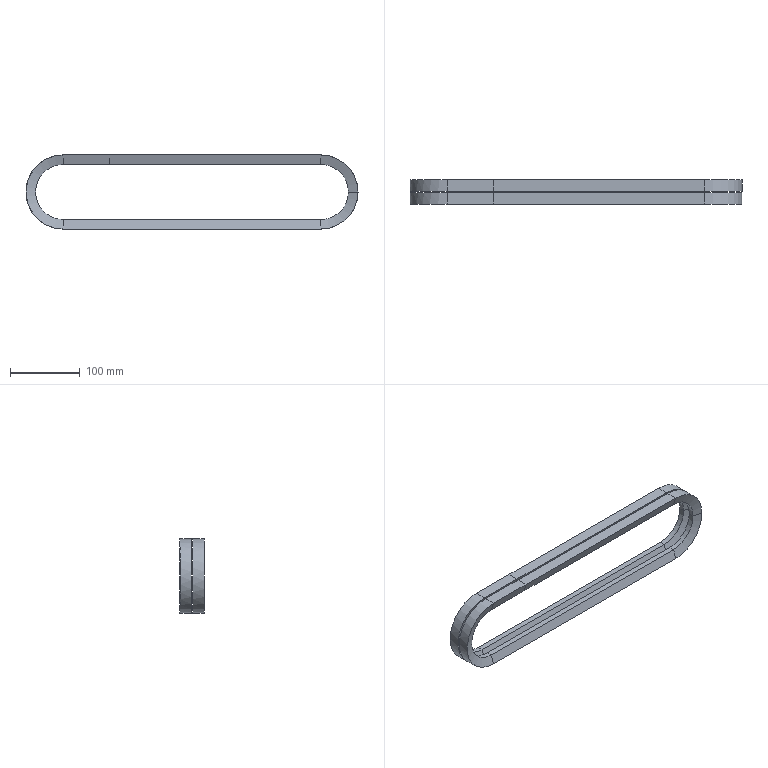Part | SolidWorks | features Sweep 1 | 2 solids | 54 faces | box 477.4 x 34.776 x 107 mm | volume 340043 mm3 | plane 27 | cone 15 | cylinder 12 | commonest cylinder face diameters 79.502 x6 106.706 x3 107 x3
STEP:
#1=CARTESIAN_POINT('',(343.918,-286.333,600.));
#2=VERTEX_POINT('',#1);
#3=CARTESIAN_POINT('',(304.166,-286.333,639.751));
#4=VERTEX_POINT('',#3);
#5=CARTESIAN_POINT('',(304.166,-286.333,600.));
#6=DIRECTION('',(0.,-1.,0.));
#7=DIRECTION('',(0.,0.,-1.));
#8=AXIS2_PLACEMENT_3D('',#5,#6,#7);
#9=CIRCLE('',#8,39.751);
#10=EDGE_CURVE('',#2,#4,#9,.T.);
#11=ORIENTED_EDGE('',*,*,#10,.F.);
#12=CARTESIAN_POINT('',(343.918,-294.066,600.));
#13=VERTEX_POINT('',#12);
#14=CARTESIAN_POINT('',(343.918,-277.7,600.));
#15=DIRECTION('',(0.,-1.,0.));
#16=VECTOR('',#15,1000.);
#17=LINE('',#14,#16);
#18=EDGE_CURVE('',#2,#13,#17,.T.);
#19=ORIENTED_EDGE('',*,*,#18,.T.);
#20=CARTESIAN_POINT('',(304.166,-294.066,639.751));
#21=VERTEX_POINT('',#20);
#22=CARTESIAN_POINT('',(304.166,-294.066,600.));
#23=DIRECTION('',(0.,-1.,0.));
#24=DIRECTION('',(0.,0.,-1.));
#25=AXIS2_PLACEMENT_3D('',#22,#23,#24);
#26=CIRCLE('',#25,39.751);
#27=EDGE_CURVE('',#13,#21,#26,.T.);
#28=ORIENTED_EDGE('',*,*,#27,.T.);
#29=CARTESIAN_POINT('',(304.166,-286.333,639.751));
#30=DIRECTION('',(0.,1.,0.));
#31=VECTOR('',#30,1000.);
#32=LINE('',#29,#31);
#33=EDGE_CURVE('',#21,#4,#32,.T.);
#34=ORIENTED_EDGE('',*,*,#33,.T.);
#35=EDGE_LOOP('',(#11,#19,#28,#34));
#36=FACE_OUTER_BOUND('',#35,.T.);
#37=CARTESIAN_POINT('',(304.166,-277.7,600.));
#38=DIRECTION('',(0.,-1.,0.));
#39=DIRECTION('',(1.,0.,0.));
#40=AXIS2_PLACEMENT_3D('',#37,#38,#39);
#41=CYLINDRICAL_SURFACE('',#40,39.751);
#42=ADVANCED_FACE('',(#36),#41,.F.);
#43=ORIENTED_EDGE('',*,*,#27,.F.);
#44=CARTESIAN_POINT('',(357.666,-298.825,600.));
#45=VERTEX_POINT('',#44);
#46=CARTESIAN_POINT('',(357.666,-298.825,600.));
#47=DIRECTION('',(0.945,-0.3271,0.));
#48=VECTOR('',#47,1000.);
#49=LINE('',#46,#48);
#50=EDGE_CURVE('',#13,#45,#49,.T.);
#51=ORIENTED_EDGE('',*,*,#50,.T.);
#52=CARTESIAN_POINT('',(304.166,-298.825,653.5));
#53=VERTEX_POINT('',#52);
#54=CARTESIAN_POINT('',(304.166,-298.825,600.));
#55=DIRECTION('',(0.,-1.,0.));
#56=DIRECTION('',(0.,0.,-1.));
#57=AXIS2_PLACEMENT_3D('',#54,#55,#56);
#58=CIRCLE('',#57,53.5);
#59=EDGE_CURVE('',#45,#53,#58,.T.);
#60=ORIENTED_EDGE('',*,*,#59,.T.);
#61=CARTESIAN_POINT('',(304.166,-294.066,639.751));
#62=DIRECTION('',(0.,0.3271,-0.945));
#63=VECTOR('',#62,1000.);
#64=LINE('',#61,#63);
#65=EDGE_CURVE('',#53,#21,#64,.T.);
#66=ORIENTED_EDGE('',*,*,#65,.T.);
#67=EDGE_LOOP('',(#43,#51,#60,#66));
#68=FACE_OUTER_BOUND('',#67,.T.);
#69=CARTESIAN_POINT('',(304.166,-298.825,600.));
#70=DIRECTION('',(0.,-1.,0.));
#71=DIRECTION('',(1.,0.,0.));
#72=AXIS2_PLACEMENT_3D('',#69,#70,#71);
#73=CONICAL_SURFACE('',#72,53.5,1.238);
#74=ADVANCED_FACE('',(#68),#73,.F.);
#75=CARTESIAN_POINT('',(304.166,-282.602,546.5));
#76=VERTEX_POINT('',#75);
#77=CARTESIAN_POINT('',(357.666,-282.602,600.));
#78=VERTEX_POINT('',#77);
#79=CARTESIAN_POINT('',(304.166,-282.602,600.));
#80=DIRECTION('',(0.,-1.,0.));
#81=DIRECTION('',(0.,0.,-1.));
#82=AXIS2_PLACEMENT_3D('',#79,#80,#81);
#83=CIRCLE('',#82,53.5);
#84=EDGE_CURVE('',#76,#78,#83,.T.);
#85=ORIENTED_EDGE('',*,*,#84,.T.);
#86=CARTESIAN_POINT('',(357.666,-277.7,600.));
#87=DIRECTION('',(0.,-1.,0.));
#88=VECTOR('',#87,1000.);
#89=LINE('',#86,#88);
#90=EDGE_CURVE('',#78,#45,#89,.T.);
#91=ORIENTED_EDGE('',*,*,#90,.T.);
#92=CARTESIAN_POINT('',(304.166,-298.825,546.5));
#93=VERTEX_POINT('',#92);
#94=CARTESIAN_POINT('',(304.166,-298.825,600.));
#95=DIRECTION('',(0.,-1.,0.));
#96=DIRECTION('',(0.,0.,-1.));
#97=AXIS2_PLACEMENT_3D('',#94,#95,#96);
#98=CIRCLE('',#97,53.5);
#99=EDGE_CURVE('',#93,#45,#98,.T.);
#100=ORIENTED_EDGE('',*,*,#99,.F.);
#101=CARTESIAN_POINT('',(304.166,-298.825,546.5));
#102=DIRECTION('',(0.,-1.,0.));
#103=VECTOR('',#102,1000.);
#104=LINE('',#101,#103);
#105=EDGE_CURVE('',#76,#93,#104,.T.);
#106=ORIENTED_EDGE('',*,*,#105,.F.);
#107=EDGE_LOOP('',(#85,#91,#100,#106));
#108=FACE_OUTER_BOUND('',#107,.T.);
#109=CARTESIAN_POINT('',(304.166,-277.7,600.));
#110=DIRECTION('',(0.,-1.,0.));
#111=DIRECTION('',(1.,0.,0.));
#112=AXIS2_PLACEMENT_3D('',#109,#110,#111);
#113=CYLINDRICAL_SURFACE('',#112,53.5);
#114=ADVANCED_FACE('',(#108),#113,.T.);
#115=CARTESIAN_POINT('',(-66.234,-282.954,652.204));
#116=VERTEX_POINT('',#115);
#117=CARTESIAN_POINT('',(-118.437,-282.954,600.));
#118=VERTEX_POINT('',#117);
#119=CARTESIAN_POINT('',(-66.234,-282.954,600.));
#120=DIRECTION('',(0.,-1.,0.));
#121=DIRECTION('',(0.,0.,1.));
#122=AXIS2_PLACEMENT_3D('',#119,#120,#121);
#123=CIRCLE('',#122,52.204);
#124=EDGE_CURVE('',#116,#118,#123,.T.);
#125=ORIENTED_EDGE('',*,*,#124,.T.);
#126=CARTESIAN_POINT('',(-119.734,-282.602,600.));
#127=VERTEX_POINT('',#126);
#128=CARTESIAN_POINT('',(-118.437,-282.954,600.));
#129=DIRECTION('',(-0.9651,0.2619,0.));
#130=VECTOR('',#129,1000.);
#131=LINE('',#128,#130);
#132=EDGE_CURVE('',#118,#127,#131,.T.);
#133=ORIENTED_EDGE('',*,*,#132,.T.);
#134=CARTESIAN_POINT('',(-66.234,-282.602,653.5));
#135=VERTEX_POINT('',#134);
#136=CARTESIAN_POINT('',(-66.234,-282.602,600.));
#137=DIRECTION('',(0.,-1.,0.));
#138=DIRECTION('',(0.,0.,1.));
#139=AXIS2_PLACEMENT_3D('',#136,#137,#138);
#140=CIRCLE('',#139,53.5);
#141=EDGE_CURVE('',#135,#127,#140,.T.);
#142=ORIENTED_EDGE('',*,*,#141,.F.);
#143=CARTESIAN_POINT('',(-66.234,-282.954,652.204));
#144=DIRECTION('',(0.,0.2619,0.9651));
#145=VECTOR('',#144,1000.);
#146=LINE('',#143,#145);
#147=EDGE_CURVE('',#116,#135,#146,.T.);
#148=ORIENTED_EDGE('',*,*,#147,.F.);
#149=EDGE_LOOP('',(#125,#133,#142,#148));
#150=FACE_OUTER_BOUND('',#149,.T.);
#151=CARTESIAN_POINT('',(-66.234,-282.954,600.));
#152=DIRECTION('',(0.,1.,0.));
#153=DIRECTION('',(-1.,0.,0.));
#154=AXIS2_PLACEMENT_3D('',#151,#152,#153);
#155=CONICAL_SURFACE('',#154,52.204,1.306);
#156=ADVANCED_FACE('',(#150),#155,.F.);
#157=CARTESIAN_POINT('',(-66.234,-286.333,639.751));
#158=VERTEX_POINT('',#157);
#159=CARTESIAN_POINT('',(-105.985,-286.333,600.));
#160=VERTEX_POINT('',#159);
#161=CARTESIAN_POINT('',(-66.234,-286.333,600.));
#162=DIRECTION('',(0.,-1.,0.));
#163=DIRECTION('',(0.,0.,1.));
#164=AXIS2_PLACEMENT_3D('',#161,#162,#163);
#165=CIRCLE('',#164,39.751);
#166=EDGE_CURVE('',#158,#160,#165,.T.);
#167=ORIENTED_EDGE('',*,*,#166,.T.);
#168=CARTESIAN_POINT('',(-105.985,-286.333,600.));
#169=DIRECTION('',(-0.9651,0.2619,0.));
#170=VECTOR('',#169,1000.);
#171=LINE('',#168,#170);
#172=EDGE_CURVE('',#160,#118,#171,.T.);
#173=ORIENTED_EDGE('',*,*,#172,.T.);
#174=ORIENTED_EDGE('',*,*,#124,.F.);
#175=CARTESIAN_POINT('',(-66.234,-282.954,652.204));
#176=DIRECTION('',(0.,0.2619,0.9651));
#177=VECTOR('',#176,1000.);
#178=LINE('',#175,#177);
#179=EDGE_CURVE('',#158,#116,#178,.T.);
#180=ORIENTED_EDGE('',*,*,#179,.F.);
#181=EDGE_LOOP('',(#167,#173,#174,#180));
#182=FACE_OUTER_BOUND('',#181,.T.);
#183=CARTESIAN_POINT('',(-66.234,-286.333,600.));
#184=DIRECTION('',(0.,1.,0.));
#185=DIRECTION('',(-1.,0.,0.));
#186=AXIS2_PLACEMENT_3D('',#183,#184,#185);
#187=CONICAL_SURFACE('',#186,39.751,1.306);
#188=ADVANCED_FACE('',(#182),#187,.F.);
#189=CARTESIAN_POINT('',(304.166,-282.602,653.5));
#190=VERTEX_POINT('',#189);
#191=CARTESIAN_POINT('',(304.166,-298.825,653.5));
#192=DIRECTION('',(0.,-1.,0.));
#193=VECTOR('',#192,1000.);
#194=LINE('',#191,#193);
#195=EDGE_CURVE('',#190,#53,#194,.T.);
#196=ORIENTED_EDGE('',*,*,#195,.F.);
#197=CARTESIAN_POINT('',(0.,-282.602,653.5));
#198=VERTEX_POINT('',#197);
#199=CARTESIAN_POINT('',(304.166,-282.602,653.5));
#200=DIRECTION('',(-1.,0.,0.));
#201=VECTOR('',#200,1000.);
#202=LINE('',#199,#201);
#203=EDGE_CURVE('',#190,#198,#202,.T.);
#204=ORIENTED_EDGE('',*,*,#203,.T.);
#205=CARTESIAN_POINT('',(0.,-298.825,653.5));
#206=VERTEX_POINT('',#205);
#207=CARTESIAN_POINT('',(0.,-298.825,653.5));
#208=DIRECTION('',(0.,-1.,0.));
#209=VECTOR('',#208,1000.);
#210=LINE('',#207,#209);
#211=EDGE_CURVE('',#198,#206,#210,.T.);
#212=ORIENTED_EDGE('',*,*,#211,.T.);
#213=CARTESIAN_POINT('',(304.166,-298.825,653.5));
#214=DIRECTION('',(-1.,0.,0.));
#215=VECTOR('',#214,1000.);
#216=LINE('',#213,#215);
#217=EDGE_CURVE('',#53,#206,#216,.T.);
#218=ORIENTED_EDGE('',*,*,#217,.F.);
#219=EDGE_LOOP('',(#196,#204,#212,#218));
#220=FACE_OUTER_BOUND('',#219,.T.);
#221=CARTESIAN_POINT('',(304.166,-298.825,653.5));
#222=DIRECTION('',(0.,0.,-1.));
#223=DIRECTION('',(-1.,0.,0.));
#224=AXIS2_PLACEMENT_3D('',#221,#222,#223);
#225=PLANE('',#224);
#226=ADVANCED_FACE('',(#220),#225,.F.);
#227=CARTESIAN_POINT('',(-66.234,-298.825,653.5));
#228=VERTEX_POINT('',#227);
#229=CARTESIAN_POINT('',(0.,-298.825,653.5));
#230=DIRECTION('',(-1.,0.,0.));
#231=VECTOR('',#230,1000.);
#232=LINE('',#229,#231);
#233=EDGE_CURVE('',#206,#228,#232,.T.);
#234=ORIENTED_EDGE('',*,*,#233,.F.);
#235=ORIENTED_EDGE('',*,*,#211,.F.);
#236=CARTESIAN_POINT('',(0.,-282.602,653.5));
#237=DIRECTION('',(-1.,0.,0.));
#238=VECTOR('',#237,1000.);
#239=LINE('',#236,#238);
#240=EDGE_CURVE('',#198,#135,#239,.T.);
#241=ORIENTED_EDGE('',*,*,#240,.T.);
#242=CARTESIAN_POINT('',(-66.234,-298.825,653.5));
#243=DIRECTION('',(0.,-1.,0.));
#244=VECTOR('',#243,1000.);
#245=LINE('',#242,#244);
#246=EDGE_CURVE('',#135,#228,#245,.T.);
#247=ORIENTED_EDGE('',*,*,#246,.T.);
#248=EDGE_LOOP('',(#234,#235,#241,#247));
#249=FACE_OUTER_BOUND('',#248,.T.);
#250=CARTESIAN_POINT('',(0.,-298.825,653.5));
#251=DIRECTION('',(0.,0.,-1.));
#252=DIRECTION('',(-1.,0.,0.));
#253=AXIS2_PLACEMENT_3D('',#250,#251,#252);
#254=PLANE('',#253);
#255=ADVANCED_FACE('',(#249),#254,.F.);
#256=CARTESIAN_POINT('',(0.,-294.066,639.751));
#257=VERTEX_POINT('',#256);
#258=CARTESIAN_POINT('',(-66.234,-294.066,639.751));
#259=VERTEX_POINT('',#258);
#260=CARTESIAN_POINT('',(0.,-294.066,639.751));
#261=DIRECTION('',(-1.,0.,0.));
#262=VECTOR('',#261,1000.);
#263=LINE('',#260,#262);
#264=EDGE_CURVE('',#257,#259,#263,.T.);
#265=ORIENTED_EDGE('',*,*,#264,.F.);
#266=CARTESIAN_POINT('',(0.,-294.066,639.751));
#267=DIRECTION('',(0.,0.3271,-0.945));
#268=VECTOR('',#267,1000.);
#269=LINE('',#266,#268);
#270=EDGE_CURVE('',#206,#257,#269,.T.);
#271=ORIENTED_EDGE('',*,*,#270,.F.);
#272=ORIENTED_EDGE('',*,*,#233,.T.);
#273=CARTESIAN_POINT('',(-66.234,-294.066,639.751));
#274=DIRECTION('',(0.,0.3271,-0.945));
#275=VECTOR('',#274,1000.);
#276=LINE('',#273,#275);
#277=EDGE_CURVE('',#228,#259,#276,.T.);
#278=ORIENTED_EDGE('',*,*,#277,.T.);
#279=EDGE_LOOP('',(#265,#271,#272,#278));
#280=FACE_OUTER_BOUND('',#279,.T.);
#281=CARTESIAN_POINT('',(0.,-294.066,639.751));
#282=DIRECTION('',(0.,0.945,0.3271));
#283=DIRECTION('',(0.,-0.3271,0.945));
#284=AXIS2_PLACEMENT_3D('',#281,#282,#283);
#285=PLANE('',#284);
#286=ADVANCED_FACE('',(#280),#285,.F.);
#287=CARTESIAN_POINT('',(0.,-286.333,639.751));
#288=VERTEX_POINT('',#287);
#289=CARTESIAN_POINT('',(0.,-286.333,639.751));
#290=DIRECTION('',(-1.,0.,0.));
#291=VECTOR('',#290,1000.);
#292=LINE('',#289,#291);
#293=EDGE_CURVE('',#288,#158,#292,.T.);
#294=ORIENTED_EDGE('',*,*,#293,.F.);
#295=CARTESIAN_POINT('',(0.,-286.333,639.751));
#296=DIRECTION('',(0.,1.,0.));
#297=VECTOR('',#296,1000.);
#298=LINE('',#295,#297);
#299=EDGE_CURVE('',#257,#288,#298,.T.);
#300=ORIENTED_EDGE('',*,*,#299,.F.);
#301=ORIENTED_EDGE('',*,*,#264,.T.);
#302=CARTESIAN_POINT('',(-66.234,-286.333,639.751));
#303=DIRECTION('',(0.,1.,0.));
#304=VECTOR('',#303,1000.);
#305=LINE('',#302,#304);
#306=EDGE_CURVE('',#259,#158,#305,.T.);
#307=ORIENTED_EDGE('',*,*,#306,.T.);
#308=EDGE_LOOP('',(#294,#300,#301,#307));
#309=FACE_OUTER_BOUND('',#308,.T.);
#310=CARTESIAN_POINT('',(0.,-286.333,639.751));
#311=DIRECTION('',(0.,0.,1.));
#312=DIRECTION('',(1.,0.,0.));
#313=AXIS2_PLACEMENT_3D('',#310,#311,#312);
#314=PLANE('',#313);
#315=ADVANCED_FACE('',(#309),#314,.F.);
#316=CARTESIAN_POINT('',(0.,-282.954,652.204));
#317=VERTEX_POINT('',#316);
#318=CARTESIAN_POINT('',(0.,-282.954,652.204));
#319=DIRECTION('',(-1.,0.,0.));
#320=VECTOR('',#319,1000.);
#321=LINE('',#318,#320);
#322=EDGE_CURVE('',#317,#116,#321,.T.);
#323=ORIENTED_EDGE('',*,*,#322,.F.);
#324=CARTESIAN_POINT('',(0.,-282.954,652.204));
#325=DIRECTION('',(0.,0.2619,0.9651));
#326=VECTOR('',#325,1000.);
#327=LINE('',#324,#326);
#328=EDGE_CURVE('',#288,#317,#327,.T.);
#329=ORIENTED_EDGE('',*,*,#328,.F.);
#330=ORIENTED_EDGE('',*,*,#293,.T.);
#331=ORIENTED_EDGE('',*,*,#179,.T.);
#332=EDGE_LOOP('',(#323,#329,#330,#331));
#333=FACE_OUTER_BOUND('',#332,.T.);
#334=CARTESIAN_POINT('',(0.,-282.954,652.204));
#335=DIRECTION('',(0.,-0.9651,0.2619));
#336=DIRECTION('',(0.,-0.2619,-0.9651));
#337=AXIS2_PLACEMENT_3D('',#334,#335,#336);
#338=PLANE('',#337);
#339=ADVANCED_FACE('',(#333),#338,.F.);
#340=ORIENTED_EDGE('',*,*,#147,.T.);
#341=ORIENTED_EDGE('',*,*,#240,.F.);
#342=CARTESIAN_POINT('',(0.,-282.954,652.204));
#343=DIRECTION('',(0.,0.2619,0.9651));
#344=VECTOR('',#343,1000.);
#345=LINE('',#342,#344);
#346=EDGE_CURVE('',#317,#198,#345,.T.);
#347=ORIENTED_EDGE('',*,*,#346,.F.);
#348=ORIENTED_EDGE('',*,*,#322,.T.);
#349=EDGE_LOOP('',(#340,#341,#347,#348));
#350=FACE_OUTER_BOUND('',#349,.T.);
#351=CARTESIAN_POINT('',(0.,-282.954,652.204));
#352=DIRECTION('',(0.,-0.9651,0.2619));
#353=DIRECTION('',(0.,-0.2619,-0.9651));
#354=AXIS2_PLACEMENT_3D('',#351,#352,#353);
#355=PLANE('',#354);
#356=ADVANCED_FACE('',(#350),#355,.F.);
#357=CARTESIAN_POINT('',(-66.234,-298.825,546.5));
#358=VERTEX_POINT('',#357);
#359=CARTESIAN_POINT('',(-66.234,-298.825,600.));
#360=DIRECTION('',(0.,-1.,0.));
#361=DIRECTION('',(0.,0.,1.));
#362=AXIS2_PLACEMENT_3D('',#359,#360,#361);
#363=CIRCLE('',#362,53.5);
#364=EDGE_CURVE('',#228,#358,#363,.T.);
#365=ORIENTED_EDGE('',*,*,#364,.F.);
#366=ORIENTED_EDGE('',*,*,#246,.F.);
#367=ORIENTED_EDGE('',*,*,#141,.T.);
#368=CARTESIAN_POINT('',(-66.234,-282.602,546.5));
#369=VERTEX_POINT('',#368);
#370=CARTESIAN_POINT('',(-66.234,-282.602,600.));
#371=DIRECTION('',(0.,-1.,0.));
#372=DIRECTION('',(0.,0.,1.));
#373=AXIS2_PLACEMENT_3D('',#370,#371,#372);
#374=CIRCLE('',#373,53.5);
#375=EDGE_CURVE('',#127,#369,#374,.T.);
#376=ORIENTED_EDGE('',*,*,#375,.T.);
#377=CARTESIAN_POINT('',(-66.234,-298.825,546.5));
#378=DIRECTION('',(0.,-1.,0.));
#379=VECTOR('',#378,1000.);
#380=LINE('',#377,#379);
#381=EDGE_CURVE('',#369,#358,#380,.T.);
#382=ORIENTED_EDGE('',*,*,#381,.T.);
#383=EDGE_LOOP('',(#365,#366,#367,#376,#382));
#384=FACE_OUTER_BOUND('',#383,.T.);
#385=CARTESIAN_POINT('',(-66.234,-277.7,600.));
#386=DIRECTION('',(0.,-1.,0.));
#387=DIRECTION('',(1.,0.,0.));
#388=AXIS2_PLACEMENT_3D('',#385,#386,#387);
#389=CYLINDRICAL_SURFACE('',#388,53.5);
#390=ADVANCED_FACE('',(#384),#389,.T.);
#391=CARTESIAN_POINT('',(-66.234,-294.066,560.249));
#392=VERTEX_POINT('',#391);
#393=CARTESIAN_POINT('',(-66.234,-294.066,600.));
#394=DIRECTION('',(0.,-1.,0.));
#395=DIRECTION('',(0.,0.,1.));
#396=AXIS2_PLACEMENT_3D('',#393,#394,#395);
#397=CIRCLE('',#396,39.751);
#398=EDGE_CURVE('',#259,#392,#397,.T.);
#399=ORIENTED_EDGE('',*,*,#398,.F.);
#400=ORIENTED_EDGE('',*,*,#277,.F.);
#401=ORIENTED_EDGE('',*,*,#364,.T.);
#402=CARTESIAN_POINT('',(-66.234,-294.066,560.249));
#403=DIRECTION('',(0.,0.3271,0.945));
#404=VECTOR('',#403,1000.);
#405=LINE('',#402,#404);
#406=EDGE_CURVE('',#358,#392,#405,.T.);
#407=ORIENTED_EDGE('',*,*,#406,.T.);
#408=EDGE_LOOP('',(#399,#400,#401,#407));
#409=FACE_OUTER_BOUND('',#408,.T.);
#410=CARTESIAN_POINT('',(-66.234,-298.825,600.));
#411=DIRECTION('',(0.,-1.,0.));
#412=DIRECTION('',(1.,0.,0.));
#413=AXIS2_PLACEMENT_3D('',#410,#411,#412);
#414=CONICAL_SURFACE('',#413,53.5,1.238);
#415=ADVANCED_FACE('',(#409),#414,.F.);
#416=ORIENTED_EDGE('',*,*,#166,.F.);
#417=ORIENTED_EDGE('',*,*,#306,.F.);
#418=ORIENTED_EDGE('',*,*,#398,.T.);
#419=CARTESIAN_POINT('',(-66.234,-286.333,560.249));
#420=VERTEX_POINT('',#419);
#421=CARTESIAN_POINT('',(-66.234,-286.333,560.249));
#422=DIRECTION('',(0.,1.,0.));
#423=VECTOR('',#422,1000.);
#424=LINE('',#421,#423);
#425=EDGE_CURVE('',#392,#420,#424,.T.);
#426=ORIENTED_EDGE('',*,*,#425,.T.);
#427=CARTESIAN_POINT('',(-66.234,-286.333,600.));
#428=DIRECTION('',(0.,-1.,0.));
#429=DIRECTION('',(0.,0.,1.));
#430=AXIS2_PLACEMENT_3D('',#427,#428,#429);
#431=CIRCLE('',#430,39.751);
#432=EDGE_CURVE('',#160,#420,#431,.T.);
#433=ORIENTED_EDGE('',*,*,#432,.F.);
#434=EDGE_LOOP('',(#416,#417,#418,#426,#433));
#435=FACE_OUTER_BOUND('',#434,.T.);
#436=CARTESIAN_POINT('',(-66.234,-277.7,600.));
#437=DIRECTION('',(0.,-1.,0.));
#438=DIRECTION('',(1.,0.,0.));
#439=AXIS2_PLACEMENT_3D('',#436,#437,#438);
#440=CYLINDRICAL_SURFACE('',#439,39.751);
#441=ADVANCED_FACE('',(#435),#440,.F.);
#442=ORIENTED_EDGE('',*,*,#172,.F.);
#443=ORIENTED_EDGE('',*,*,#432,.T.);
#444=CARTESIAN_POINT('',(-66.234,-282.954,547.796));
#445=VERTEX_POINT('',#444);
#446=CARTESIAN_POINT('',(-66.234,-282.954,547.796));
#447=DIRECTION('',(0.,0.2619,-0.9651));
#448=VECTOR('',#447,1000.);
#449=LINE('',#446,#448);
#450=EDGE_CURVE('',#420,#445,#449,.T.);
#451=ORIENTED_EDGE('',*,*,#450,.T.);
#452=CARTESIAN_POINT('',(-66.234,-282.954,600.));
#453=DIRECTION('',(0.,-1.,0.));
#454=DIRECTION('',(0.,0.,1.));
#455=AXIS2_PLACEMENT_3D('',#452,#453,#454);
#456=CIRCLE('',#455,52.204);
#457=EDGE_CURVE('',#118,#445,#456,.T.);
#458=ORIENTED_EDGE('',*,*,#457,.F.);
#459=EDGE_LOOP('',(#442,#443,#451,#458));
#460=FACE_OUTER_BOUND('',#459,.T.);
#461=CARTESIAN_POINT('',(-66.234,-286.333,600.));
#462=DIRECTION('',(0.,1.,0.));
#463=DIRECTION('',(-1.,0.,0.));
#464=AXIS2_PLACEMENT_3D('',#461,#462,#463);
#465=CONICAL_SURFACE('',#464,39.751,1.306);
#466=ADVANCED_FACE('',(#460),#465,.F.);
#467=ORIENTED_EDGE('',*,*,#132,.F.);
#468=ORIENTED_EDGE('',*,*,#457,.T.);
#469=CARTESIAN_POINT('',(-66.234,-282.954,547.796));
#470=DIRECTION('',(0.,0.2619,-0.9651));
#471=VECTOR('',#470,1000.);
#472=LINE('',#469,#471);
#473=EDGE_CURVE('',#445,#369,#472,.T.);
#474=ORIENTED_EDGE('',*,*,#473,.T.);
#475=ORIENTED_EDGE('',*,*,#375,.F.);
#476=EDGE_LOOP('',(#467,#468,#474,#475));
#477=FACE_OUTER_BOUND('',#476,.T.);
#478=CARTESIAN_POINT('',(-66.234,-282.954,600.));
#479=DIRECTION('',(0.,1.,0.));
#480=DIRECTION('',(-1.,0.,0.));
#481=AXIS2_PLACEMENT_3D('',#478,#479,#480);
#482=CONICAL_SURFACE('',#481,52.204,1.306);
#483=ADVANCED_FACE('',(#477),#482,.F.);
#484=CARTESIAN_POINT('',(-66.234,-298.825,546.5));
#485=DIRECTION('',(1.,0.,0.));
#486=VECTOR('',#485,1000.);
#487=LINE('',#484,#486);
#488=EDGE_CURVE('',#358,#93,#487,.T.);
#489=ORIENTED_EDGE('',*,*,#488,.F.);
#490=ORIENTED_EDGE('',*,*,#381,.F.);
#491=CARTESIAN_POINT('',(-66.234,-282.602,546.5));
#492=DIRECTION('',(1.,0.,0.));
#493=VECTOR('',#492,1000.);
#494=LINE('',#491,#493);
#495=EDGE_CURVE('',#369,#76,#494,.T.);
#496=ORIENTED_EDGE('',*,*,#495,.T.);
#497=ORIENTED_EDGE('',*,*,#105,.T.);
#498=EDGE_LOOP('',(#489,#490,#496,#497));
#499=FACE_OUTER_BOUND('',#498,.T.);
#500=CARTESIAN_POINT('',(-66.234,-298.825,546.5));
#501=DIRECTION('',(0.,0.,1.));
#502=DIRECTION('',(0.,-1.,0.));
#503=AXIS2_PLACEMENT_3D('',#500,#501,#502);
#504=PLANE('',#503);
#505=ADVANCED_FACE('',(#499),#504,.F.);
#506=CARTESIAN_POINT('',(304.166,-294.066,560.249));
#507=VERTEX_POINT('',#506);
#508=CARTESIAN_POINT('',(-66.234,-294.066,560.249));
#509=DIRECTION('',(1.,0.,0.));
#510=VECTOR('',#509,1000.);
#511=LINE('',#508,#510);
#512=EDGE_CURVE('',#392,#507,#511,.T.);
#513=ORIENTED_EDGE('',*,*,#512,.F.);
#514=ORIENTED_EDGE('',*,*,#406,.F.);
#515=ORIENTED_EDGE('',*,*,#488,.T.);
#516=CARTESIAN_POINT('',(304.166,-294.066,560.249));
#517=DIRECTION('',(0.,0.3271,0.945));
#518=VECTOR('',#517,1000.);
#519=LINE('',#516,#518);
#520=EDGE_CURVE('',#93,#507,#519,.T.);
#521=ORIENTED_EDGE('',*,*,#520,.T.);
#522=EDGE_LOOP('',(#513,#514,#515,#521));
#523=FACE_OUTER_BOUND('',#522,.T.);
#524=CARTESIAN_POINT('',(-66.234,-294.066,560.249));
#525=DIRECTION('',(0.,0.945,-0.3271));
#526=DIRECTION('',(0.,0.3271,0.945));
#527=AXIS2_PLACEMENT_3D('',#524,#525,#526);
#528=PLANE('',#527);
#529=ADVANCED_FACE('',(#523),#528,.F.);
#530=CARTESIAN_POINT('',(304.166,-286.333,560.249));
#531=VERTEX_POINT('',#530);
#532=CARTESIAN_POINT('',(-66.234,-286.333,560.249));
#533=DIRECTION('',(1.,0.,0.));
#534=VECTOR('',#533,1000.);
#535=LINE('',#532,#534);
#536=EDGE_CURVE('',#420,#531,#535,.T.);
#537=ORIENTED_EDGE('',*,*,#536,.F.);
#538=ORIENTED_EDGE('',*,*,#425,.F.);
#539=ORIENTED_EDGE('',*,*,#512,.T.);
#540=CARTESIAN_POINT('',(304.166,-286.333,560.249));
#541=DIRECTION('',(0.,1.,0.));
#542=VECTOR('',#541,1000.);
#543=LINE('',#540,#542);
#544=EDGE_CURVE('',#507,#531,#543,.T.);
#545=ORIENTED_EDGE('',*,*,#544,.T.);
#546=EDGE_LOOP('',(#537,#538,#539,#545));
#547=FACE_OUTER_BOUND('',#546,.T.);
#548=CARTESIAN_POINT('',(-66.234,-286.333,560.249));
#549=DIRECTION('',(0.,0.,-1.));
#550=DIRECTION('',(0.,1.,0.));
#551=AXIS2_PLACEMENT_3D('',#548,#549,#550);
#552=PLANE('',#551);
#553=ADVANCED_FACE('',(#547),#552,.F.);
#554=CARTESIAN_POINT('',(304.166,-282.954,547.796));
#555=VERTEX_POINT('',#554);
#556=CARTESIAN_POINT('',(-66.234,-282.954,547.796));
#557=DIRECTION('',(1.,0.,0.));
#558=VECTOR('',#557,1000.);
#559=LINE('',#556,#558);
#560=EDGE_CURVE('',#445,#555,#559,.T.);
#561=ORIENTED_EDGE('',*,*,#560,.F.);
#562=ORIENTED_EDGE('',*,*,#450,.F.);
#563=ORIENTED_EDGE('',*,*,#536,.T.);
#564=CARTESIAN_POINT('',(304.166,-282.954,547.796));
#565=DIRECTION('',(0.,0.2619,-0.9651));
#566=VECTOR('',#565,1000.);
#567=LINE('',#564,#566);
#568=EDGE_CURVE('',#531,#555,#567,.T.);
#569=ORIENTED_EDGE('',*,*,#568,.T.);
#570=EDGE_LOOP('',(#561,#562,#563,#569));
#571=FACE_OUTER_BOUND('',#570,.T.);
#572=CARTESIAN_POINT('',(-66.234,-282.954,547.796));
#573=DIRECTION('',(0.,-0.9651,-0.2619));
#574=DIRECTION('',(0.,0.2619,-0.9651));
#575=AXIS2_PLACEMENT_3D('',#572,#573,#574);
#576=PLANE('',#575);
#577=ADVANCED_FACE('',(#571),#576,.F.);
#578=CARTESIAN_POINT('',(304.166,-282.954,547.796));
#579=DIRECTION('',(0.,0.2619,-0.9651));
#580=VECTOR('',#579,1000.);
#581=LINE('',#578,#580);
#582=EDGE_CURVE('',#555,#76,#581,.T.);
#583=ORIENTED_EDGE('',*,*,#582,.T.);
#584=ORIENTED_EDGE('',*,*,#495,.F.);
#585=ORIENTED_EDGE('',*,*,#473,.F.);
#586=ORIENTED_EDGE('',*,*,#560,.T.);
#587=EDGE_LOOP('',(#583,#584,#585,#586));
#588=FACE_OUTER_BOUND('',#587,.T.);
#589=CARTESIAN_POINT('',(-66.234,-282.954,547.796));
#590=DIRECTION('',(0.,-0.9651,-0.2619));
#591=DIRECTION('',(0.,0.2619,-0.9651));
#592=AXIS2_PLACEMENT_3D('',#589,#590,#591);
#593=PLANE('',#592);
#594=ADVANCED_FACE('',(#588),#593,.F.);
#595=ORIENTED_EDGE('',*,*,#90,.F.);
#596=CARTESIAN_POINT('',(304.166,-282.602,600.));
#597=DIRECTION('',(0.,-1.,0.));
#598=DIRECTION('',(0.,0.,-1.));
#599=AXIS2_PLACEMENT_3D('',#596,#597,#598);
#600=CIRCLE('',#599,53.5);
#601=EDGE_CURVE('',#78,#190,#600,.T.);
#602=ORIENTED_EDGE('',*,*,#601,.T.);
#603=ORIENTED_EDGE('',*,*,#195,.T.);
#604=ORIENTED_EDGE('',*,*,#59,.F.);
#605=EDGE_LOOP('',(#595,#602,#603,#604));
#606=FACE_OUTER_BOUND('',#605,.T.);
#607=CARTESIAN_POINT('',(304.166,-277.7,600.));
#608=DIRECTION('',(0.,-1.,0.));
#609=DIRECTION('',(1.,0.,0.));
#610=AXIS2_PLACEMENT_3D('',#607,#608,#609);
#611=CYLINDRICAL_SURFACE('',#610,53.5);
#612=ADVANCED_FACE('',(#606),#611,.T.);
#613=ORIENTED_EDGE('',*,*,#50,.F.);
#614=CARTESIAN_POINT('',(304.166,-294.066,600.));
#615=DIRECTION('',(0.,-1.,0.));
#616=DIRECTION('',(0.,0.,-1.));
#617=AXIS2_PLACEMENT_3D('',#614,#615,#616);
#618=CIRCLE('',#617,39.751);
#619=EDGE_CURVE('',#507,#13,#618,.T.);
#620=ORIENTED_EDGE('',*,*,#619,.F.);
#621=ORIENTED_EDGE('',*,*,#520,.F.);
#622=ORIENTED_EDGE('',*,*,#99,.T.);
#623=EDGE_LOOP('',(#613,#620,#621,#622));
#624=FACE_OUTER_BOUND('',#623,.T.);
#625=CARTESIAN_POINT('',(304.166,-298.825,600.));
#626=DIRECTION('',(0.,-1.,0.));
#627=DIRECTION('',(1.,0.,0.));
#628=AXIS2_PLACEMENT_3D('',#625,#626,#627);
#629=CONICAL_SURFACE('',#628,53.5,1.238);
#630=ADVANCED_FACE('',(#624),#629,.F.);
#631=ORIENTED_EDGE('',*,*,#18,.F.);
#632=CARTESIAN_POINT('',(304.166,-286.333,600.));
#633=DIRECTION('',(0.,-1.,0.));
#634=DIRECTION('',(0.,0.,-1.));
#635=AXIS2_PLACEMENT_3D('',#632,#633,#634);
#636=CIRCLE('',#635,39.751);
#637=EDGE_CURVE('',#531,#2,#636,.T.);
#638=ORIENTED_EDGE('',*,*,#637,.F.);
#639=ORIENTED_EDGE('',*,*,#544,.F.);
#640=ORIENTED_EDGE('',*,*,#619,.T.);
#641=EDGE_LOOP('',(#631,#638,#639,#640));
#642=FACE_OUTER_BOUND('',#641,.T.);
#643=CARTESIAN_POINT('',(304.166,-277.7,600.));
#644=DIRECTION('',(0.,-1.,0.));
#645=DIRECTION('',(1.,0.,0.));
#646=AXIS2_PLACEMENT_3D('',#643,#644,#645);
#647=CYLINDRICAL_SURFACE('',#646,39.751);
#648=ADVANCED_FACE('',(#642),#647,.F.);
#649=CARTESIAN_POINT('',(304.166,-282.954,652.204));
#650=VERTEX_POINT('',#649);
#651=CARTESIAN_POINT('',(304.166,-282.954,600.));
#652=DIRECTION('',(0.,-1.,0.));
#653=DIRECTION('',(0.,0.,-1.));
#654=AXIS2_PLACEMENT_3D('',#651,#652,#653);
#655=CIRCLE('',#654,52.204);
#656=EDGE_CURVE('',#555,#650,#655,.T.);
#657=ORIENTED_EDGE('',*,*,#656,.F.);
#658=ORIENTED_EDGE('',*,*,#568,.F.);
#659=ORIENTED_EDGE('',*,*,#637,.T.);
#660=ORIENTED_EDGE('',*,*,#10,.T.);
#661=CARTESIAN_POINT('',(304.166,-282.954,652.204));
#662=DIRECTION('',(0.,0.2619,0.9651));
#663=VECTOR('',#662,1000.);
#664=LINE('',#661,#663);
#665=EDGE_CURVE('',#4,#650,#664,.T.);
#666=ORIENTED_EDGE('',*,*,#665,.T.);
#667=EDGE_LOOP('',(#657,#658,#659,#660,#666));
#668=FACE_OUTER_BOUND('',#667,.T.);
#669=CARTESIAN_POINT('',(304.166,-286.333,600.));
#670=DIRECTION('',(0.,1.,0.));
#671=DIRECTION('',(-1.,0.,0.));
#672=AXIS2_PLACEMENT_3D('',#669,#670,#671);
#673=CONICAL_SURFACE('',#672,39.751,1.306);
#674=ADVANCED_FACE('',(#668),#673,.F.);
#675=CARTESIAN_POINT('',(304.166,-282.954,652.204));
#676=DIRECTION('',(0.,0.2619,0.9651));
#677=VECTOR('',#676,1000.);
#678=LINE('',#675,#677);
#679=EDGE_CURVE('',#650,#190,#678,.T.);
#680=ORIENTED_EDGE('',*,*,#679,.T.);
#681=ORIENTED_EDGE('',*,*,#601,.F.);
#682=ORIENTED_EDGE('',*,*,#84,.F.);
#683=ORIENTED_EDGE('',*,*,#582,.F.);
#684=ORIENTED_EDGE('',*,*,#656,.T.);
#685=EDGE_LOOP('',(#680,#681,#682,#683,#684));
#686=FACE_OUTER_BOUND('',#685,.T.);
#687=CARTESIAN_POINT('',(304.166,-282.954,600.));
#688=DIRECTION('',(0.,1.,0.));
#689=DIRECTION('',(-1.,0.,0.));
#690=AXIS2_PLACEMENT_3D('',#687,#688,#689);
#691=CONICAL_SURFACE('',#690,52.204,1.306);
#692=ADVANCED_FACE('',(#686),#691,.F.);
#693=ORIENTED_EDGE('',*,*,#217,.T.);
#694=ORIENTED_EDGE('',*,*,#270,.T.);
#695=CARTESIAN_POINT('',(304.166,-294.066,639.751));
#696=DIRECTION('',(-1.,0.,0.));
#697=VECTOR('',#696,1000.);
#698=LINE('',#695,#697);
#699=EDGE_CURVE('',#21,#257,#698,.T.);
#700=ORIENTED_EDGE('',*,*,#699,.F.);
#701=ORIENTED_EDGE('',*,*,#65,.F.);
#702=EDGE_LOOP('',(#693,#694,#700,#701));
#703=FACE_OUTER_BOUND('',#702,.T.);
#704=CARTESIAN_POINT('',(304.166,-294.066,639.751));
#705=DIRECTION('',(0.,0.945,0.3271));
#706=DIRECTION('',(0.,-0.3271,0.945));
#707=AXIS2_PLACEMENT_3D('',#704,#705,#706);
#708=PLANE('',#707);
#709=ADVANCED_FACE('',(#703),#708,.F.);
#710=ORIENTED_EDGE('',*,*,#699,.T.);
#711=ORIENTED_EDGE('',*,*,#299,.T.);
#712=CARTESIAN_POINT('',(304.166,-286.333,639.751));
#713=DIRECTION('',(-1.,0.,0.));
#714=VECTOR('',#713,1000.);
#715=LINE('',#712,#714);
#716=EDGE_CURVE('',#4,#288,#715,.T.);
#717=ORIENTED_EDGE('',*,*,#716,.F.);
#718=ORIENTED_EDGE('',*,*,#33,.F.);
#719=EDGE_LOOP('',(#710,#711,#717,#718));
#720=FACE_OUTER_BOUND('',#719,.T.);
#721=CARTESIAN_POINT('',(304.166,-286.333,639.751));
#722=DIRECTION('',(0.,0.,1.));
#723=DIRECTION('',(1.,0.,0.));
#724=AXIS2_PLACEMENT_3D('',#721,#722,#723);
#725=PLANE('',#724);
#726=ADVANCED_FACE('',(#720),#725,.F.);
#727=ORIENTED_EDGE('',*,*,#716,.T.);
#728=ORIENTED_EDGE('',*,*,#328,.T.);
#729=CARTESIAN_POINT('',(304.166,-282.954,652.204));
#730=DIRECTION('',(-1.,0.,0.));
#731=VECTOR('',#730,1000.);
#732=LINE('',#729,#731);
#733=EDGE_CURVE('',#650,#317,#732,.T.);
#734=ORIENTED_EDGE('',*,*,#733,.F.);
#735=ORIENTED_EDGE('',*,*,#665,.F.);
#736=EDGE_LOOP('',(#727,#728,#734,#735));
#737=FACE_OUTER_BOUND('',#736,.T.);
#738=CARTESIAN_POINT('',(304.166,-282.954,652.204));
#739=DIRECTION('',(0.,-0.9651,0.2619));
#740=DIRECTION('',(0.,-0.2619,-0.9651));
#741=AXIS2_PLACEMENT_3D('',#738,#739,#740);
#742=PLANE('',#741);
#743=ADVANCED_FACE('',(#737),#742,.F.);
#744=ORIENTED_EDGE('',*,*,#733,.T.);
#745=ORIENTED_EDGE('',*,*,#346,.T.);
#746=ORIENTED_EDGE('',*,*,#203,.F.);
#747=ORIENTED_EDGE('',*,*,#679,.F.);
#748=EDGE_LOOP('',(#744,#745,#746,#747));
#749=FACE_OUTER_BOUND('',#748,.T.);
#750=CARTESIAN_POINT('',(304.166,-282.954,652.204));
#751=DIRECTION('',(0.,-0.9651,0.2619));
#752=DIRECTION('',(0.,-0.2619,-0.9651));
#753=AXIS2_PLACEMENT_3D('',#750,#751,#752);
#754=PLANE('',#753);
#755=ADVANCED_FACE('',(#749),#754,.F.);
#756=CLOSED_SHELL('',(#42,#74,#114,#156,#188,#226,#255,#286,#315,#339,#356,#390,#415,#441,#466,#483,#505,#529,#553,#577,#594,#612,#630,#648,#674,#692,#709,#726,#743,#755));
#757=MANIFOLD_SOLID_BREP('',#756);
#758=CARTESIAN_POINT('',(304.166,-301.185,546.647));
#759=VERTEX_POINT('',#758);
#760=CARTESIAN_POINT('',(357.519,-301.185,600.));
#761=VERTEX_POINT('',#760);
#762=CARTESIAN_POINT('',(304.166,-301.185,600.));
#763=DIRECTION('',(0.,-1.,0.));
#764=DIRECTION('',(0.,0.,-1.));
#765=AXIS2_PLACEMENT_3D('',#762,#763,#764);
#766=CIRCLE('',#765,53.353);
#767=EDGE_CURVE('',#759,#761,#766,.T.);
#768=ORIENTED_EDGE('',*,*,#767,.T.);
#769=CARTESIAN_POINT('',(357.519,-317.379,600.));
#770=VERTEX_POINT('',#769);
#771=CARTESIAN_POINT('',(357.519,-277.7,600.));
#772=DIRECTION('',(0.,-1.,0.));
#773=VECTOR('',#772,1000.);
#774=LINE('',#771,#773);
#775=EDGE_CURVE('',#761,#770,#774,.T.);
#776=ORIENTED_EDGE('',*,*,#775,.T.);
#777=CARTESIAN_POINT('',(304.166,-317.379,546.647));
#778=VERTEX_POINT('',#777);
#779=CARTESIAN_POINT('',(304.166,-317.379,600.));
#780=DIRECTION('',(0.,-1.,0.));
#781=DIRECTION('',(0.,0.,-1.));
#782=AXIS2_PLACEMENT_3D('',#779,#780,#781);
#783=CIRCLE('',#782,53.353);
#784=EDGE_CURVE('',#778,#770,#783,.T.);
#785=ORIENTED_EDGE('',*,*,#784,.F.);
#786=CARTESIAN_POINT('',(304.166,-317.379,546.647));
#787=DIRECTION('',(0.,-1.,0.));
#788=VECTOR('',#787,1000.);
#789=LINE('',#786,#788);
#790=EDGE_CURVE('',#759,#778,#789,.T.);
#791=ORIENTED_EDGE('',*,*,#790,.F.);
#792=EDGE_LOOP('',(#768,#776,#785,#791));
#793=FACE_OUTER_BOUND('',#792,.T.);
#794=CARTESIAN_POINT('',(304.166,-277.7,600.));
#795=DIRECTION('',(0.,-1.,0.));
#796=DIRECTION('',(1.,0.,0.));
#797=AXIS2_PLACEMENT_3D('',#794,#795,#796);
#798=CYLINDRICAL_SURFACE('',#797,53.353);
#799=ADVANCED_FACE('',(#793),#798,.T.);
#800=CARTESIAN_POINT('',(343.918,-305.333,600.));
#801=VERTEX_POINT('',#800);
#802=CARTESIAN_POINT('',(304.166,-305.333,639.751));
#803=VERTEX_POINT('',#802);
#804=CARTESIAN_POINT('',(304.166,-305.333,600.));
#805=DIRECTION('',(0.,-1.,0.));
#806=DIRECTION('',(0.,0.,-1.));
#807=AXIS2_PLACEMENT_3D('',#804,#805,#806);
#808=CIRCLE('',#807,39.751);
#809=EDGE_CURVE('',#801,#803,#808,.T.);
#810=ORIENTED_EDGE('',*,*,#809,.F.);
#811=CARTESIAN_POINT('',(343.918,-313.066,600.));
#812=VERTEX_POINT('',#811);
#813=CARTESIAN_POINT('',(343.918,-277.7,600.));
#814=DIRECTION('',(0.,-1.,0.));
#815=VECTOR('',#814,1000.);
#816=LINE('',#813,#815);
#817=EDGE_CURVE('',#801,#812,#816,.T.);
#818=ORIENTED_EDGE('',*,*,#817,.T.);
#819=CARTESIAN_POINT('',(304.166,-313.066,639.751));
#820=VERTEX_POINT('',#819);
#821=CARTESIAN_POINT('',(304.166,-313.066,600.));
#822=DIRECTION('',(0.,-1.,0.));
#823=DIRECTION('',(0.,0.,-1.));
#824=AXIS2_PLACEMENT_3D('',#821,#822,#823);
#825=CIRCLE('',#824,39.751);
#826=EDGE_CURVE('',#812,#820,#825,.T.);
#827=ORIENTED_EDGE('',*,*,#826,.T.);
#828=CARTESIAN_POINT('',(304.166,-305.333,639.751));
#829=DIRECTION('',(0.,1.,0.));
#830=VECTOR('',#829,1000.);
#831=LINE('',#828,#830);
#832=EDGE_CURVE('',#820,#803,#831,.T.);
#833=ORIENTED_EDGE('',*,*,#832,.T.);
#834=EDGE_LOOP('',(#810,#818,#827,#833));
#835=FACE_OUTER_BOUND('',#834,.T.);
#836=CARTESIAN_POINT('',(304.166,-277.7,600.));
#837=DIRECTION('',(0.,-1.,0.));
#838=DIRECTION('',(1.,0.,0.));
#839=AXIS2_PLACEMENT_3D('',#836,#837,#838);
#840=CYLINDRICAL_SURFACE('',#839,39.751);
#841=ADVANCED_FACE('',(#835),#840,.F.);
#842=ORIENTED_EDGE('',*,*,#826,.F.);
#843=CARTESIAN_POINT('',(357.519,-317.379,600.));
#844=DIRECTION('',(0.9532,-0.3022,0.));
#845=VECTOR('',#844,1000.);
#846=LINE('',#843,#845);
#847=EDGE_CURVE('',#812,#770,#846,.T.);
#848=ORIENTED_EDGE('',*,*,#847,.T.);
#849=CARTESIAN_POINT('',(304.166,-317.379,653.353));
#850=VERTEX_POINT('',#849);
#851=CARTESIAN_POINT('',(304.166,-317.379,600.));
#852=DIRECTION('',(0.,-1.,0.));
#853=DIRECTION('',(0.,0.,-1.));
#854=AXIS2_PLACEMENT_3D('',#851,#852,#853);
#855=CIRCLE('',#854,53.353);
#856=EDGE_CURVE('',#770,#850,#855,.T.);
#857=ORIENTED_EDGE('',*,*,#856,.T.);
#858=CARTESIAN_POINT('',(304.166,-313.066,639.751));
#859=DIRECTION('',(0.,0.3022,-0.9532));
#860=VECTOR('',#859,1000.);
#861=LINE('',#858,#860);
#862=EDGE_CURVE('',#850,#820,#861,.T.);
#863=ORIENTED_EDGE('',*,*,#862,.T.);
#864=EDGE_LOOP('',(#842,#848,#857,#863));
#865=FACE_OUTER_BOUND('',#864,.T.);
#866=CARTESIAN_POINT('',(304.166,-317.379,600.));
#867=DIRECTION('',(0.,-1.,0.));
#868=DIRECTION('',(1.,0.,0.));
#869=AXIS2_PLACEMENT_3D('',#866,#867,#868);
#870=CONICAL_SURFACE('',#869,53.353,1.264);
#871=ADVANCED_FACE('',(#865),#870,.F.);
#872=CARTESIAN_POINT('',(-66.234,-305.333,639.751));
#873=VERTEX_POINT('',#872);
#874=CARTESIAN_POINT('',(-105.985,-305.333,600.));
#875=VERTEX_POINT('',#874);
#876=CARTESIAN_POINT('',(-66.234,-305.333,600.));
#877=DIRECTION('',(0.,-1.,0.));
#878=DIRECTION('',(0.,0.,1.));
#879=AXIS2_PLACEMENT_3D('',#876,#877,#878);
#880=CIRCLE('',#879,39.751);
#881=EDGE_CURVE('',#873,#875,#880,.T.);
#882=ORIENTED_EDGE('',*,*,#881,.T.);
#883=CARTESIAN_POINT('',(-119.586,-301.185,600.));
#884=VERTEX_POINT('',#883);
#885=CARTESIAN_POINT('',(-105.985,-305.333,600.));
#886=DIRECTION('',(-0.9565,0.2917,0.));
#887=VECTOR('',#886,1000.);
#888=LINE('',#885,#887);
#889=EDGE_CURVE('',#875,#884,#888,.T.);
#890=ORIENTED_EDGE('',*,*,#889,.T.);
#891=CARTESIAN_POINT('',(-66.234,-301.185,653.353));
#892=VERTEX_POINT('',#891);
#893=CARTESIAN_POINT('',(-66.234,-301.185,600.));
#894=DIRECTION('',(0.,-1.,0.));
#895=DIRECTION('',(0.,0.,1.));
#896=AXIS2_PLACEMENT_3D('',#893,#894,#895);
#897=CIRCLE('',#896,53.353);
#898=EDGE_CURVE('',#892,#884,#897,.T.);
#899=ORIENTED_EDGE('',*,*,#898,.F.);
#900=CARTESIAN_POINT('',(-66.234,-301.185,653.353));
#901=DIRECTION('',(0.,0.2917,0.9565));
#902=VECTOR('',#901,1000.);
#903=LINE('',#900,#902);
#904=EDGE_CURVE('',#873,#892,#903,.T.);
#905=ORIENTED_EDGE('',*,*,#904,.F.);
#906=EDGE_LOOP('',(#882,#890,#899,#905));
#907=FACE_OUTER_BOUND('',#906,.T.);
#908=CARTESIAN_POINT('',(-66.234,-305.333,600.));
#909=DIRECTION('',(0.,1.,0.));
#910=DIRECTION('',(-1.,0.,0.));
#911=AXIS2_PLACEMENT_3D('',#908,#909,#910);
#912=CONICAL_SURFACE('',#911,39.751,1.275);
#913=ADVANCED_FACE('',(#907),#912,.F.);
#914=ORIENTED_EDGE('',*,*,#862,.F.);
#915=CARTESIAN_POINT('',(0.,-317.379,653.353));
#916=VERTEX_POINT('',#915);
#917=CARTESIAN_POINT('',(304.166,-317.379,653.353));
#918=DIRECTION('',(-1.,0.,0.));
#919=VECTOR('',#918,1000.);
#920=LINE('',#917,#919);
#921=EDGE_CURVE('',#850,#916,#920,.T.);
#922=ORIENTED_EDGE('',*,*,#921,.T.);
#923=CARTESIAN_POINT('',(0.,-313.066,639.751));
#924=VERTEX_POINT('',#923);
#925=CARTESIAN_POINT('',(0.,-313.066,639.751));
#926=DIRECTION('',(0.,0.3022,-0.9532));
#927=VECTOR('',#926,1000.);
#928=LINE('',#925,#927);
#929=EDGE_CURVE('',#916,#924,#928,.T.);
#930=ORIENTED_EDGE('',*,*,#929,.T.);
#931=CARTESIAN_POINT('',(304.166,-313.066,639.751));
#932=DIRECTION('',(-1.,0.,0.));
#933=VECTOR('',#932,1000.);
#934=LINE('',#931,#933);
#935=EDGE_CURVE('',#820,#924,#934,.T.);
#936=ORIENTED_EDGE('',*,*,#935,.F.);
#937=EDGE_LOOP('',(#914,#922,#930,#936));
#938=FACE_OUTER_BOUND('',#937,.T.);
#939=CARTESIAN_POINT('',(304.166,-313.066,639.751));
#940=DIRECTION('',(0.,0.9532,0.3022));
#941=DIRECTION('',(0.,-0.3022,0.9532));
#942=AXIS2_PLACEMENT_3D('',#939,#940,#941);
#943=PLANE('',#942);
#944=ADVANCED_FACE('',(#938),#943,.F.);
#945=CARTESIAN_POINT('',(-66.234,-313.066,639.751));
#946=VERTEX_POINT('',#945);
#947=CARTESIAN_POINT('',(0.,-313.066,639.751));
#948=DIRECTION('',(-1.,0.,0.));
#949=VECTOR('',#948,1000.);
#950=LINE('',#947,#949);
#951=EDGE_CURVE('',#924,#946,#950,.T.);
#952=ORIENTED_EDGE('',*,*,#951,.F.);
#953=ORIENTED_EDGE('',*,*,#929,.F.);
#954=CARTESIAN_POINT('',(-66.234,-317.379,653.353));
#955=VERTEX_POINT('',#954);
#956=CARTESIAN_POINT('',(0.,-317.379,653.353));
#957=DIRECTION('',(-1.,0.,0.));
#958=VECTOR('',#957,1000.);
#959=LINE('',#956,#958);
#960=EDGE_CURVE('',#916,#955,#959,.T.);
#961=ORIENTED_EDGE('',*,*,#960,.T.);
#962=CARTESIAN_POINT('',(-66.234,-313.066,639.751));
#963=DIRECTION('',(0.,0.3022,-0.9532));
#964=VECTOR('',#963,1000.);
#965=LINE('',#962,#964);
#966=EDGE_CURVE('',#955,#946,#965,.T.);
#967=ORIENTED_EDGE('',*,*,#966,.T.);
#968=EDGE_LOOP('',(#952,#953,#961,#967));
#969=FACE_OUTER_BOUND('',#968,.T.);
#970=CARTESIAN_POINT('',(0.,-313.066,639.751));
#971=DIRECTION('',(0.,0.9532,0.3022));
#972=DIRECTION('',(0.,-0.3022,0.9532));
#973=AXIS2_PLACEMENT_3D('',#970,#971,#972);
#974=PLANE('',#973);
#975=ADVANCED_FACE('',(#969),#974,.F.);
#976=CARTESIAN_POINT('',(0.,-305.333,639.751));
#977=VERTEX_POINT('',#976);
#978=CARTESIAN_POINT('',(0.,-305.333,639.751));
#979=DIRECTION('',(-1.,0.,0.));
#980=VECTOR('',#979,1000.);
#981=LINE('',#978,#980);
#982=EDGE_CURVE('',#977,#873,#981,.T.);
#983=ORIENTED_EDGE('',*,*,#982,.F.);
#984=CARTESIAN_POINT('',(0.,-305.333,639.751));
#985=DIRECTION('',(0.,1.,0.));
#986=VECTOR('',#985,1000.);
#987=LINE('',#984,#986);
#988=EDGE_CURVE('',#924,#977,#987,.T.);
#989=ORIENTED_EDGE('',*,*,#988,.F.);
#990=ORIENTED_EDGE('',*,*,#951,.T.);
#991=CARTESIAN_POINT('',(-66.234,-305.333,639.751));
#992=DIRECTION('',(0.,1.,0.));
#993=VECTOR('',#992,1000.);
#994=LINE('',#991,#993);
#995=EDGE_CURVE('',#946,#873,#994,.T.);
#996=ORIENTED_EDGE('',*,*,#995,.T.);
#997=EDGE_LOOP('',(#983,#989,#990,#996));
#998=FACE_OUTER_BOUND('',#997,.T.);
#999=CARTESIAN_POINT('',(0.,-305.333,639.751));
#1000=DIRECTION('',(0.,0.,1.));
#1001=DIRECTION('',(1.,0.,0.));
#1002=AXIS2_PLACEMENT_3D('',#999,#1000,#1001);
#1003=PLANE('',#1002);
#1004=ADVANCED_FACE('',(#998),#1003,.F.);
#1005=CARTESIAN_POINT('',(0.,-301.185,653.353));
#1006=VERTEX_POINT('',#1005);
#1007=CARTESIAN_POINT('',(0.,-301.185,653.353));
#1008=DIRECTION('',(-1.,0.,0.));
#1009=VECTOR('',#1008,1000.);
#1010=LINE('',#1007,#1009);
#1011=EDGE_CURVE('',#1006,#892,#1010,.T.);
#1012=ORIENTED_EDGE('',*,*,#1011,.F.);
#1013=CARTESIAN_POINT('',(0.,-301.185,653.353));
#1014=DIRECTION('',(0.,0.2917,0.9565));
#1015=VECTOR('',#1014,1000.);
#1016=LINE('',#1013,#1015);
#1017=EDGE_CURVE('',#977,#1006,#1016,.T.);
#1018=ORIENTED_EDGE('',*,*,#1017,.F.);
#1019=ORIENTED_EDGE('',*,*,#982,.T.);
#1020=ORIENTED_EDGE('',*,*,#904,.T.);
#1021=EDGE_LOOP('',(#1012,#1018,#1019,#1020));
#1022=FACE_OUTER_BOUND('',#1021,.T.);
#1023=CARTESIAN_POINT('',(0.,-301.185,653.353));
#1024=DIRECTION('',(0.,-0.9565,0.2917));
#1025=DIRECTION('',(0.,-0.2917,-0.9565));
#1026=AXIS2_PLACEMENT_3D('',#1023,#1024,#1025);
#1027=PLANE('',#1026);
#1028=ADVANCED_FACE('',(#1022),#1027,.F.);
#1029=CARTESIAN_POINT('',(-66.234,-317.379,653.353));
#1030=DIRECTION('',(0.,-1.,0.));
#1031=VECTOR('',#1030,1000.);
#1032=LINE('',#1029,#1031);
#1033=EDGE_CURVE('',#892,#955,#1032,.T.);
#1034=ORIENTED_EDGE('',*,*,#1033,.T.);
#1035=ORIENTED_EDGE('',*,*,#960,.F.);
#1036=CARTESIAN_POINT('',(0.,-317.379,653.353));
#1037=DIRECTION('',(0.,-1.,0.));
#1038=VECTOR('',#1037,1000.);
#1039=LINE('',#1036,#1038);
#1040=EDGE_CURVE('',#1006,#916,#1039,.T.);
#1041=ORIENTED_EDGE('',*,*,#1040,.F.);
#1042=ORIENTED_EDGE('',*,*,#1011,.T.);
#1043=EDGE_LOOP('',(#1034,#1035,#1041,#1042));
#1044=FACE_OUTER_BOUND('',#1043,.T.);
#1045=CARTESIAN_POINT('',(0.,-317.379,653.353));
#1046=DIRECTION('',(0.,0.,-1.));
#1047=DIRECTION('',(-1.,0.,0.));
#1048=AXIS2_PLACEMENT_3D('',#1045,#1046,#1047);
#1049=PLANE('',#1048);
#1050=ADVANCED_FACE('',(#1044),#1049,.F.);
#1051=CARTESIAN_POINT('',(-66.234,-313.066,560.249));
#1052=VERTEX_POINT('',#1051);
#1053=CARTESIAN_POINT('',(-66.234,-313.066,600.));
#1054=DIRECTION('',(0.,-1.,0.));
#1055=DIRECTION('',(0.,0.,1.));
#1056=AXIS2_PLACEMENT_3D('',#1053,#1054,#1055);
#1057=CIRCLE('',#1056,39.751);
#1058=EDGE_CURVE('',#946,#1052,#1057,.T.);
#1059=ORIENTED_EDGE('',*,*,#1058,.F.);
#1060=ORIENTED_EDGE('',*,*,#966,.F.);
#1061=CARTESIAN_POINT('',(-66.234,-317.379,546.647));
#1062=VERTEX_POINT('',#1061);
#1063=CARTESIAN_POINT('',(-66.234,-317.379,600.));
#1064=DIRECTION('',(0.,-1.,0.));
#1065=DIRECTION('',(0.,0.,1.));
#1066=AXIS2_PLACEMENT_3D('',#1063,#1064,#1065);
#1067=CIRCLE('',#1066,53.353);
#1068=EDGE_CURVE('',#955,#1062,#1067,.T.);
#1069=ORIENTED_EDGE('',*,*,#1068,.T.);
#1070=CARTESIAN_POINT('',(-66.234,-313.066,560.249));
#1071=DIRECTION('',(0.,0.3022,0.9532));
#1072=VECTOR('',#1071,1000.);
#1073=LINE('',#1070,#1072);
#1074=EDGE_CURVE('',#1062,#1052,#1073,.T.);
#1075=ORIENTED_EDGE('',*,*,#1074,.T.);
#1076=EDGE_LOOP('',(#1059,#1060,#1069,#1075));
#1077=FACE_OUTER_BOUND('',#1076,.T.);
#1078=CARTESIAN_POINT('',(-66.234,-317.379,600.));
#1079=DIRECTION('',(0.,-1.,0.));
#1080=DIRECTION('',(1.,0.,0.));
#1081=AXIS2_PLACEMENT_3D('',#1078,#1079,#1080);
#1082=CONICAL_SURFACE('',#1081,53.353,1.264);
#1083=ADVANCED_FACE('',(#1077),#1082,.F.);
#1084=ORIENTED_EDGE('',*,*,#881,.F.);
#1085=ORIENTED_EDGE('',*,*,#995,.F.);
#1086=ORIENTED_EDGE('',*,*,#1058,.T.);
#1087=CARTESIAN_POINT('',(-66.234,-305.333,560.249));
#1088=VERTEX_POINT('',#1087);
#1089=CARTESIAN_POINT('',(-66.234,-305.333,560.249));
#1090=DIRECTION('',(0.,1.,0.));
#1091=VECTOR('',#1090,1000.);
#1092=LINE('',#1089,#1091);
#1093=EDGE_CURVE('',#1052,#1088,#1092,.T.);
#1094=ORIENTED_EDGE('',*,*,#1093,.T.);
#1095=CARTESIAN_POINT('',(-66.234,-305.333,600.));
#1096=DIRECTION('',(0.,-1.,0.));
#1097=DIRECTION('',(0.,0.,1.));
#1098=AXIS2_PLACEMENT_3D('',#1095,#1096,#1097);
#1099=CIRCLE('',#1098,39.751);
#1100=EDGE_CURVE('',#875,#1088,#1099,.T.);
#1101=ORIENTED_EDGE('',*,*,#1100,.F.);
#1102=EDGE_LOOP('',(#1084,#1085,#1086,#1094,#1101));
#1103=FACE_OUTER_BOUND('',#1102,.T.);
#1104=CARTESIAN_POINT('',(-66.234,-277.7,600.));
#1105=DIRECTION('',(0.,-1.,0.));
#1106=DIRECTION('',(1.,0.,0.));
#1107=AXIS2_PLACEMENT_3D('',#1104,#1105,#1106);
#1108=CYLINDRICAL_SURFACE('',#1107,39.751);
#1109=ADVANCED_FACE('',(#1103),#1108,.F.);
#1110=ORIENTED_EDGE('',*,*,#889,.F.);
#1111=ORIENTED_EDGE('',*,*,#1100,.T.);
#1112=CARTESIAN_POINT('',(-66.234,-301.185,546.647));
#1113=VERTEX_POINT('',#1112);
#1114=CARTESIAN_POINT('',(-66.234,-301.185,546.647));
#1115=DIRECTION('',(0.,0.2917,-0.9565));
#1116=VECTOR('',#1115,1000.);
#1117=LINE('',#1114,#1116);
#1118=EDGE_CURVE('',#1088,#1113,#1117,.T.);
#1119=ORIENTED_EDGE('',*,*,#1118,.T.);
#1120=CARTESIAN_POINT('',(-66.234,-301.185,600.));
#1121=DIRECTION('',(0.,-1.,0.));
#1122=DIRECTION('',(0.,0.,1.));
#1123=AXIS2_PLACEMENT_3D('',#1120,#1121,#1122);
#1124=CIRCLE('',#1123,53.353);
#1125=EDGE_CURVE('',#884,#1113,#1124,.T.);
#1126=ORIENTED_EDGE('',*,*,#1125,.F.);
#1127=EDGE_LOOP('',(#1110,#1111,#1119,#1126));
#1128=FACE_OUTER_BOUND('',#1127,.T.);
#1129=CARTESIAN_POINT('',(-66.234,-305.333,600.));
#1130=DIRECTION('',(0.,1.,0.));
#1131=DIRECTION('',(-1.,0.,0.));
#1132=AXIS2_PLACEMENT_3D('',#1129,#1130,#1131);
#1133=CONICAL_SURFACE('',#1132,39.751,1.275);
#1134=ADVANCED_FACE('',(#1128),#1133,.F.);
#1135=CARTESIAN_POINT('',(-66.234,-317.379,546.647));
#1136=DIRECTION('',(0.,-1.,0.));
#1137=VECTOR('',#1136,1000.);
#1138=LINE('',#1135,#1137);
#1139=EDGE_CURVE('',#1113,#1062,#1138,.T.);
#1140=ORIENTED_EDGE('',*,*,#1139,.T.);
#1141=ORIENTED_EDGE('',*,*,#1068,.F.);
#1142=ORIENTED_EDGE('',*,*,#1033,.F.);
#1143=ORIENTED_EDGE('',*,*,#898,.T.);
#1144=ORIENTED_EDGE('',*,*,#1125,.T.);
#1145=EDGE_LOOP('',(#1140,#1141,#1142,#1143,#1144));
#1146=FACE_OUTER_BOUND('',#1145,.T.);
#1147=CARTESIAN_POINT('',(-66.234,-277.7,600.));
#1148=DIRECTION('',(0.,-1.,0.));
#1149=DIRECTION('',(1.,0.,0.));
#1150=AXIS2_PLACEMENT_3D('',#1147,#1148,#1149);
#1151=CYLINDRICAL_SURFACE('',#1150,53.353);
#1152=ADVANCED_FACE('',(#1146),#1151,.T.);
#1153=CARTESIAN_POINT('',(304.166,-313.066,560.249));
#1154=VERTEX_POINT('',#1153);
#1155=CARTESIAN_POINT('',(-66.234,-313.066,560.249));
#1156=DIRECTION('',(1.,0.,0.));
#1157=VECTOR('',#1156,1000.);
#1158=LINE('',#1155,#1157);
#1159=EDGE_CURVE('',#1052,#1154,#1158,.T.);
#1160=ORIENTED_EDGE('',*,*,#1159,.F.);
#1161=ORIENTED_EDGE('',*,*,#1074,.F.);
#1162=CARTESIAN_POINT('',(-66.234,-317.379,546.647));
#1163=DIRECTION('',(1.,0.,0.));
#1164=VECTOR('',#1163,1000.);
#1165=LINE('',#1162,#1164);
#1166=EDGE_CURVE('',#1062,#778,#1165,.T.);
#1167=ORIENTED_EDGE('',*,*,#1166,.T.);
#1168=CARTESIAN_POINT('',(304.166,-313.066,560.249));
#1169=DIRECTION('',(0.,0.3022,0.9532));
#1170=VECTOR('',#1169,1000.);
#1171=LINE('',#1168,#1170);
#1172=EDGE_CURVE('',#778,#1154,#1171,.T.);
#1173=ORIENTED_EDGE('',*,*,#1172,.T.);
#1174=EDGE_LOOP('',(#1160,#1161,#1167,#1173));
#1175=FACE_OUTER_BOUND('',#1174,.T.);
#1176=CARTESIAN_POINT('',(-66.234,-313.066,560.249));
#1177=DIRECTION('',(0.,0.9532,-0.3022));
#1178=DIRECTION('',(0.,0.3022,0.9532));
#1179=AXIS2_PLACEMENT_3D('',#1176,#1177,#1178);
#1180=PLANE('',#1179);
#1181=ADVANCED_FACE('',(#1175),#1180,.F.);
#1182=CARTESIAN_POINT('',(304.166,-305.333,560.249));
#1183=VERTEX_POINT('',#1182);
#1184=CARTESIAN_POINT('',(-66.234,-305.333,560.249));
#1185=DIRECTION('',(1.,0.,0.));
#1186=VECTOR('',#1185,1000.);
#1187=LINE('',#1184,#1186);
#1188=EDGE_CURVE('',#1088,#1183,#1187,.T.);
#1189=ORIENTED_EDGE('',*,*,#1188,.F.);
#1190=ORIENTED_EDGE('',*,*,#1093,.F.);
#1191=ORIENTED_EDGE('',*,*,#1159,.T.);
#1192=CARTESIAN_POINT('',(304.166,-305.333,560.249));
#1193=DIRECTION('',(0.,1.,0.));
#1194=VECTOR('',#1193,1000.);
#1195=LINE('',#1192,#1194);
#1196=EDGE_CURVE('',#1154,#1183,#1195,.T.);
#1197=ORIENTED_EDGE('',*,*,#1196,.T.);
#1198=EDGE_LOOP('',(#1189,#1190,#1191,#1197));
#1199=FACE_OUTER_BOUND('',#1198,.T.);
#1200=CARTESIAN_POINT('',(-66.234,-305.333,560.249));
#1201=DIRECTION('',(0.,0.,-1.));
#1202=DIRECTION('',(0.,1.,0.));
#1203=AXIS2_PLACEMENT_3D('',#1200,#1201,#1202);
#1204=PLANE('',#1203);
#1205=ADVANCED_FACE('',(#1199),#1204,.F.);
#1206=CARTESIAN_POINT('',(-66.234,-301.185,546.647));
#1207=DIRECTION('',(1.,0.,0.));
#1208=VECTOR('',#1207,1000.);
#1209=LINE('',#1206,#1208);
#1210=EDGE_CURVE('',#1113,#759,#1209,.T.);
#1211=ORIENTED_EDGE('',*,*,#1210,.F.);
#1212=ORIENTED_EDGE('',*,*,#1118,.F.);
#1213=ORIENTED_EDGE('',*,*,#1188,.T.);
#1214=CARTESIAN_POINT('',(304.166,-301.185,546.647));
#1215=DIRECTION('',(0.,0.2917,-0.9565));
#1216=VECTOR('',#1215,1000.);
#1217=LINE('',#1214,#1216);
#1218=EDGE_CURVE('',#1183,#759,#1217,.T.);
#1219=ORIENTED_EDGE('',*,*,#1218,.T.);
#1220=EDGE_LOOP('',(#1211,#1212,#1213,#1219));
#1221=FACE_OUTER_BOUND('',#1220,.T.);
#1222=CARTESIAN_POINT('',(-66.234,-301.185,546.647));
#1223=DIRECTION('',(0.,-0.9565,-0.2917));
#1224=DIRECTION('',(0.,0.2917,-0.9565));
#1225=AXIS2_PLACEMENT_3D('',#1222,#1223,#1224);
#1226=PLANE('',#1225);
#1227=ADVANCED_FACE('',(#1221),#1226,.F.);
#1228=ORIENTED_EDGE('',*,*,#790,.T.);
#1229=ORIENTED_EDGE('',*,*,#1166,.F.);
#1230=ORIENTED_EDGE('',*,*,#1139,.F.);
#1231=ORIENTED_EDGE('',*,*,#1210,.T.);
#1232=EDGE_LOOP('',(#1228,#1229,#1230,#1231));
#1233=FACE_OUTER_BOUND('',#1232,.T.);
#1234=CARTESIAN_POINT('',(-66.234,-317.379,546.647));
#1235=DIRECTION('',(0.,0.,1.));
#1236=DIRECTION('',(0.,-1.,0.));
#1237=AXIS2_PLACEMENT_3D('',#1234,#1235,#1236);
#1238=PLANE('',#1237);
#1239=ADVANCED_FACE('',(#1233),#1238,.F.);
#1240=ORIENTED_EDGE('',*,*,#847,.F.);
#1241=CARTESIAN_POINT('',(304.166,-313.066,600.));
#1242=DIRECTION('',(0.,-1.,0.));
#1243=DIRECTION('',(0.,0.,-1.));
#1244=AXIS2_PLACEMENT_3D('',#1241,#1242,#1243);
#1245=CIRCLE('',#1244,39.751);
#1246=EDGE_CURVE('',#1154,#812,#1245,.T.);
#1247=ORIENTED_EDGE('',*,*,#1246,.F.);
#1248=ORIENTED_EDGE('',*,*,#1172,.F.);
#1249=ORIENTED_EDGE('',*,*,#784,.T.);
#1250=EDGE_LOOP('',(#1240,#1247,#1248,#1249));
#1251=FACE_OUTER_BOUND('',#1250,.T.);
#1252=CARTESIAN_POINT('',(304.166,-317.379,600.));
#1253=DIRECTION('',(0.,-1.,0.));
#1254=DIRECTION('',(1.,0.,0.));
#1255=AXIS2_PLACEMENT_3D('',#1252,#1253,#1254);
#1256=CONICAL_SURFACE('',#1255,53.353,1.264);
#1257=ADVANCED_FACE('',(#1251),#1256,.F.);
#1258=ORIENTED_EDGE('',*,*,#817,.F.);
#1259=CARTESIAN_POINT('',(304.166,-305.333,600.));
#1260=DIRECTION('',(0.,-1.,0.));
#1261=DIRECTION('',(0.,0.,-1.));
#1262=AXIS2_PLACEMENT_3D('',#1259,#1260,#1261);
#1263=CIRCLE('',#1262,39.751);
#1264=EDGE_CURVE('',#1183,#801,#1263,.T.);
#1265=ORIENTED_EDGE('',*,*,#1264,.F.);
#1266=ORIENTED_EDGE('',*,*,#1196,.F.);
#1267=ORIENTED_EDGE('',*,*,#1246,.T.);
#1268=EDGE_LOOP('',(#1258,#1265,#1266,#1267));
#1269=FACE_OUTER_BOUND('',#1268,.T.);
#1270=CARTESIAN_POINT('',(304.166,-277.7,600.));
#1271=DIRECTION('',(0.,-1.,0.));
#1272=DIRECTION('',(1.,0.,0.));
#1273=AXIS2_PLACEMENT_3D('',#1270,#1271,#1272);
#1274=CYLINDRICAL_SURFACE('',#1273,39.751);
#1275=ADVANCED_FACE('',(#1269),#1274,.F.);
#1276=ORIENTED_EDGE('',*,*,#767,.F.);
#1277=ORIENTED_EDGE('',*,*,#1218,.F.);
#1278=ORIENTED_EDGE('',*,*,#1264,.T.);
#1279=ORIENTED_EDGE('',*,*,#809,.T.);
#1280=CARTESIAN_POINT('',(304.166,-301.185,653.353));
#1281=VERTEX_POINT('',#1280);
#1282=CARTESIAN_POINT('',(304.166,-301.185,653.353));
#1283=DIRECTION('',(0.,0.2917,0.9565));
#1284=VECTOR('',#1283,1000.);
#1285=LINE('',#1282,#1284);
#1286=EDGE_CURVE('',#803,#1281,#1285,.T.);
#1287=ORIENTED_EDGE('',*,*,#1286,.T.);
#1288=CARTESIAN_POINT('',(304.166,-301.185,600.));
#1289=DIRECTION('',(0.,-1.,0.));
#1290=DIRECTION('',(0.,0.,-1.));
#1291=AXIS2_PLACEMENT_3D('',#1288,#1289,#1290);
#1292=CIRCLE('',#1291,53.353);
#1293=EDGE_CURVE('',#761,#1281,#1292,.T.);
#1294=ORIENTED_EDGE('',*,*,#1293,.F.);
#1295=EDGE_LOOP('',(#1276,#1277,#1278,#1279,#1287,#1294));
#1296=FACE_OUTER_BOUND('',#1295,.T.);
#1297=CARTESIAN_POINT('',(304.166,-305.333,600.));
#1298=DIRECTION('',(0.,1.,0.));
#1299=DIRECTION('',(-1.,0.,0.));
#1300=AXIS2_PLACEMENT_3D('',#1297,#1298,#1299);
#1301=CONICAL_SURFACE('',#1300,39.751,1.275);
#1302=ADVANCED_FACE('',(#1296),#1301,.F.);
#1303=ORIENTED_EDGE('',*,*,#775,.F.);
#1304=ORIENTED_EDGE('',*,*,#1293,.T.);
#1305=CARTESIAN_POINT('',(304.166,-317.379,653.353));
#1306=DIRECTION('',(0.,-1.,0.));
#1307=VECTOR('',#1306,1000.);
#1308=LINE('',#1305,#1307);
#1309=EDGE_CURVE('',#1281,#850,#1308,.T.);
#1310=ORIENTED_EDGE('',*,*,#1309,.T.);
#1311=ORIENTED_EDGE('',*,*,#856,.F.);
#1312=EDGE_LOOP('',(#1303,#1304,#1310,#1311));
#1313=FACE_OUTER_BOUND('',#1312,.T.);
#1314=CARTESIAN_POINT('',(304.166,-277.7,600.));
#1315=DIRECTION('',(0.,-1.,0.));
#1316=DIRECTION('',(1.,0.,0.));
#1317=AXIS2_PLACEMENT_3D('',#1314,#1315,#1316);
#1318=CYLINDRICAL_SURFACE('',#1317,53.353);
#1319=ADVANCED_FACE('',(#1313),#1318,.T.);
#1320=ORIENTED_EDGE('',*,*,#935,.T.);
#1321=ORIENTED_EDGE('',*,*,#988,.T.);
#1322=CARTESIAN_POINT('',(304.166,-305.333,639.751));
#1323=DIRECTION('',(-1.,0.,0.));
#1324=VECTOR('',#1323,1000.);
#1325=LINE('',#1322,#1324);
#1326=EDGE_CURVE('',#803,#977,#1325,.T.);
#1327=ORIENTED_EDGE('',*,*,#1326,.F.);
#1328=ORIENTED_EDGE('',*,*,#832,.F.);
#1329=EDGE_LOOP('',(#1320,#1321,#1327,#1328));
#1330=FACE_OUTER_BOUND('',#1329,.T.);
#1331=CARTESIAN_POINT('',(304.166,-305.333,639.751));
#1332=DIRECTION('',(0.,0.,1.));
#1333=DIRECTION('',(1.,0.,0.));
#1334=AXIS2_PLACEMENT_3D('',#1331,#1332,#1333);
#1335=PLANE('',#1334);
#1336=ADVANCED_FACE('',(#1330),#1335,.F.);
#1337=ORIENTED_EDGE('',*,*,#1326,.T.);
#1338=ORIENTED_EDGE('',*,*,#1017,.T.);
#1339=CARTESIAN_POINT('',(304.166,-301.185,653.353));
#1340=DIRECTION('',(-1.,0.,0.));
#1341=VECTOR('',#1340,1000.);
#1342=LINE('',#1339,#1341);
#1343=EDGE_CURVE('',#1281,#1006,#1342,.T.);
#1344=ORIENTED_EDGE('',*,*,#1343,.F.);
#1345=ORIENTED_EDGE('',*,*,#1286,.F.);
#1346=EDGE_LOOP('',(#1337,#1338,#1344,#1345));
#1347=FACE_OUTER_BOUND('',#1346,.T.);
#1348=CARTESIAN_POINT('',(304.166,-301.185,653.353));
#1349=DIRECTION('',(0.,-0.9565,0.2917));
#1350=DIRECTION('',(0.,-0.2917,-0.9565));
#1351=AXIS2_PLACEMENT_3D('',#1348,#1349,#1350);
#1352=PLANE('',#1351);
#1353=ADVANCED_FACE('',(#1347),#1352,.F.);
#1354=ORIENTED_EDGE('',*,*,#1343,.T.);
#1355=ORIENTED_EDGE('',*,*,#1040,.T.);
#1356=ORIENTED_EDGE('',*,*,#921,.F.);
#1357=ORIENTED_EDGE('',*,*,#1309,.F.);
#1358=EDGE_LOOP('',(#1354,#1355,#1356,#1357));
#1359=FACE_OUTER_BOUND('',#1358,.T.);
#1360=CARTESIAN_POINT('',(304.166,-317.379,653.353));
#1361=DIRECTION('',(0.,0.,-1.));
#1362=DIRECTION('',(-1.,0.,0.));
#1363=AXIS2_PLACEMENT_3D('',#1360,#1361,#1362);
#1364=PLANE('',#1363);
#1365=ADVANCED_FACE('',(#1359),#1364,.F.);
#1366=CLOSED_SHELL('',(#799,#841,#871,#913,#944,#975,#1004,#1028,#1050,#1083,#1109,#1134,#1152,#1181,#1205,#1227,#1239,#1257,#1275,#1302,#1319,#1336,#1353,#1365));
#1367=MANIFOLD_SOLID_BREP('',#1366);
#1368=CARTESIAN_POINT('',(0.,0.,0.));
#1369=DIRECTION('',(0.,0.,1.));
#1370=DIRECTION('',(1.,0.,0.));
#1371=AXIS2_PLACEMENT_3D('',#1368,#1369,#1370);
#1372=(LENGTH_UNIT()NAMED_UNIT(*)SI_UNIT(.MILLI.,.METRE.));
#1373=UNCERTAINTY_MEASURE_WITH_UNIT(LENGTH_MEASURE(0.00001),#1372,'','');
#1374=(NAMED_UNIT(*)PLANE_ANGLE_UNIT()SI_UNIT($,.RADIAN.));
#1375=(NAMED_UNIT(*)SI_UNIT($,.STERADIAN.)SOLID_ANGLE_UNIT());
#1376=(GEOMETRIC_REPRESENTATION_CONTEXT(3)GLOBAL_UNCERTAINTY_ASSIGNED_CONTEXT((#1373))GLOBAL_UNIT_ASSIGNED_CONTEXT((#1372,#1374,#1375))REPRESENTATION_CONTEXT('',''));
#1377=ADVANCED_BREP_SHAPE_REPRESENTATION('',(#757,#1367,#1371),#1376);